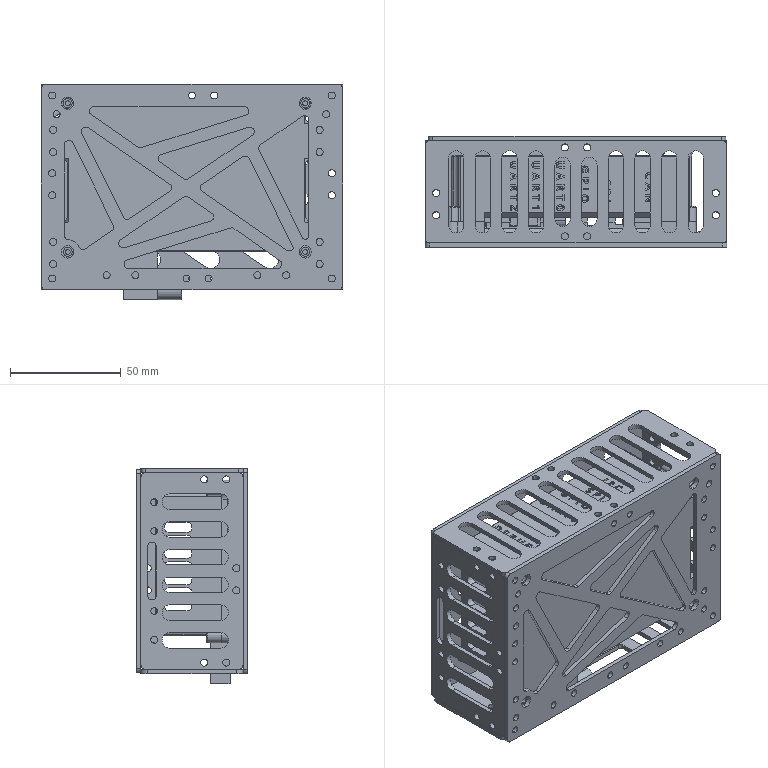Part | SolidWorks | 9 solids | 1620 faces | box 136 x 50 x 97 mm | volume 125770 mm3 | plane 766 | cylinder 586 | spline 236 | cone 20 | sphere 8 | torus 4 | commonest cylinder face diameters 3.2 x148 7 x83 4 x63 2 x59 4.5 x32 8 x30